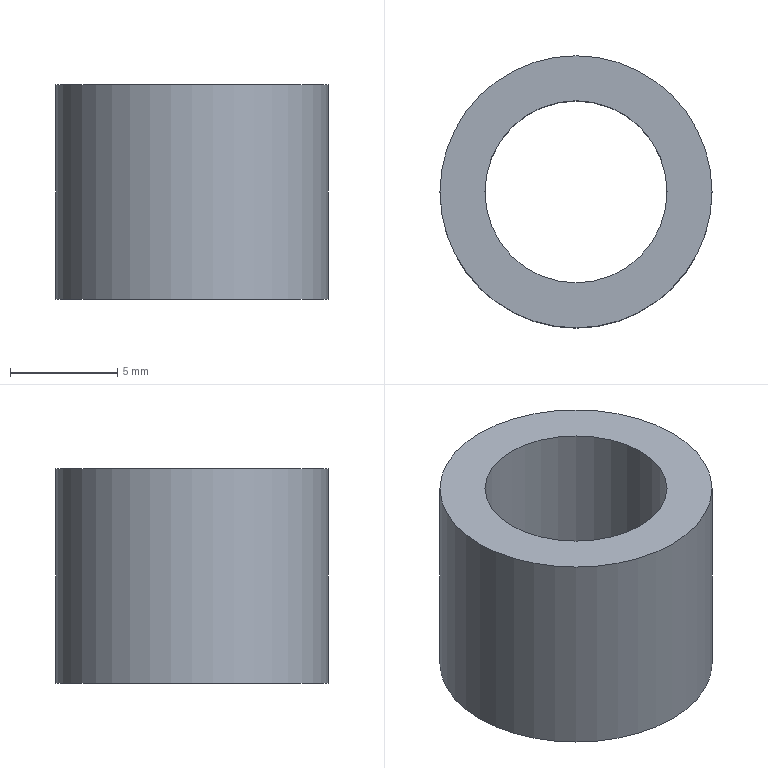Part | STEP file | 5091205 | 1 solid | 4 faces | box 12.7 x 12.7 x 10 mm | volume 699.319 mm3 | plane 2 | cylinder 2 | commonest cylinder face diameters 8.5 x1 12.7 x1
STEP:
#1=CARTESIAN_POINT('',(0.,0.,0.));
#2=DIRECTION('',(0.,0.,1.));
#3=DIRECTION('',(1.,0.,0.));
#4=AXIS2_PLACEMENT_3D('',#1,#2,#3);
#5=CARTESIAN_POINT('',(6.35,0.,5.));
#6=VERTEX_POINT('',#5);
#7=CARTESIAN_POINT('',(0.,0.,5.));
#8=DIRECTION('',(0.,0.,1.));
#9=DIRECTION('',(1.,0.,0.));
#10=AXIS2_PLACEMENT_3D('',#7,#8,#9);
#11=CIRCLE('',#10,6.35);
#12=CARTESIAN_POINT('',(0.,0.,5.));
#13=DIRECTION('',(0.,0.,1.));
#14=DIRECTION('',(1.,0.,0.));
#15=AXIS2_PLACEMENT_3D('',#12,#13,#14);
#16=PLANE('',#15);
#17=CARTESIAN_POINT('',(0.,0.));
#18=DIRECTION('',(1.,0.));
#19=AXIS2_PLACEMENT_2D('',#17,#18);
#20=CIRCLE('',#19,6.35);
#21=(GEOMETRIC_REPRESENTATION_CONTEXT(2)PARAMETRIC_REPRESENTATION_CONTEXT()REPRESENTATION_CONTEXT('',''));
#22=DEFINITIONAL_REPRESENTATION('',(#20),#21);
#23=PCURVE('',#16,#22);
#24=CARTESIAN_POINT('',(0.,0.,5.));
#25=DIRECTION('',(0.,0.,-1.));
#26=DIRECTION('',(-1.,0.,0.));
#27=AXIS2_PLACEMENT_3D('',#24,#25,#26);
#28=CYLINDRICAL_SURFACE('',#27,6.35);
#29=CARTESIAN_POINT('',(9.425,0.));
#30=DIRECTION('',(-1.,0.));
#31=VECTOR('',#30,1.);
#32=LINE('',#29,#31);
#33=(GEOMETRIC_REPRESENTATION_CONTEXT(2)PARAMETRIC_REPRESENTATION_CONTEXT()REPRESENTATION_CONTEXT('',''));
#34=DEFINITIONAL_REPRESENTATION('',(#32),#33);
#35=PCURVE('',#28,#34);
#36=SURFACE_CURVE('',#11,(#23,#35),.PCURVE_S1.);
#37=EDGE_CURVE('',#6,#6,#36,.T.);
#38=ORIENTED_EDGE('',*,*,#37,.T.);
#39=EDGE_LOOP('',(#38));
#40=FACE_BOUND('',#39,.T.);
#41=CARTESIAN_POINT('',(4.25,0.,5.));
#42=VERTEX_POINT('',#41);
#43=CARTESIAN_POINT('',(0.,0.,5.));
#44=DIRECTION('',(0.,0.,1.));
#45=DIRECTION('',(1.,0.,0.));
#46=AXIS2_PLACEMENT_3D('',#43,#44,#45);
#47=CIRCLE('',#46,4.25);
#48=CARTESIAN_POINT('',(0.,0.));
#49=DIRECTION('',(1.,0.));
#50=AXIS2_PLACEMENT_2D('',#48,#49);
#51=CIRCLE('',#50,4.25);
#52=(GEOMETRIC_REPRESENTATION_CONTEXT(2)PARAMETRIC_REPRESENTATION_CONTEXT()REPRESENTATION_CONTEXT('',''));
#53=DEFINITIONAL_REPRESENTATION('',(#51),#52);
#54=PCURVE('',#16,#53);
#55=CARTESIAN_POINT('',(0.,0.,5.));
#56=DIRECTION('',(0.,0.,-1.));
#57=DIRECTION('',(-1.,0.,0.));
#58=AXIS2_PLACEMENT_3D('',#55,#56,#57);
#59=CYLINDRICAL_SURFACE('',#58,4.25);
#60=CARTESIAN_POINT('',(9.425,0.));
#61=DIRECTION('',(-1.,0.));
#62=VECTOR('',#61,1.);
#63=LINE('',#60,#62);
#64=(GEOMETRIC_REPRESENTATION_CONTEXT(2)PARAMETRIC_REPRESENTATION_CONTEXT()REPRESENTATION_CONTEXT('',''));
#65=DEFINITIONAL_REPRESENTATION('',(#63),#64);
#66=PCURVE('',#59,#65);
#67=SURFACE_CURVE('',#47,(#54,#66),.PCURVE_S1.);
#68=EDGE_CURVE('',#42,#42,#67,.T.);
#69=ORIENTED_EDGE('',*,*,#68,.F.);
#70=EDGE_LOOP('',(#69));
#71=FACE_BOUND('',#70,.T.);
#72=ADVANCED_FACE('',(#40,#71),#16,.T.);
#73=CARTESIAN_POINT('',(6.35,0.,-5.));
#74=VERTEX_POINT('',#73);
#75=CARTESIAN_POINT('',(0.,0.,-5.));
#76=DIRECTION('',(0.,0.,1.));
#77=DIRECTION('',(1.,0.,0.));
#78=AXIS2_PLACEMENT_3D('',#75,#76,#77);
#79=CIRCLE('',#78,6.35);
#80=CARTESIAN_POINT('',(0.,0.,-5.));
#81=DIRECTION('',(0.,0.,1.));
#82=DIRECTION('',(1.,0.,0.));
#83=AXIS2_PLACEMENT_3D('',#80,#81,#82);
#84=PLANE('',#83);
#85=CARTESIAN_POINT('',(0.,0.));
#86=DIRECTION('',(1.,0.));
#87=AXIS2_PLACEMENT_2D('',#85,#86);
#88=CIRCLE('',#87,6.35);
#89=(GEOMETRIC_REPRESENTATION_CONTEXT(2)PARAMETRIC_REPRESENTATION_CONTEXT()REPRESENTATION_CONTEXT('',''));
#90=DEFINITIONAL_REPRESENTATION('',(#88),#89);
#91=PCURVE('',#84,#90);
#92=CARTESIAN_POINT('',(9.425,10.));
#93=DIRECTION('',(-1.,0.));
#94=VECTOR('',#93,1.);
#95=LINE('',#92,#94);
#96=(GEOMETRIC_REPRESENTATION_CONTEXT(2)PARAMETRIC_REPRESENTATION_CONTEXT()REPRESENTATION_CONTEXT('',''));
#97=DEFINITIONAL_REPRESENTATION('',(#95),#96);
#98=PCURVE('',#28,#97);
#99=SURFACE_CURVE('',#79,(#91,#98),.PCURVE_S1.);
#100=EDGE_CURVE('',#74,#74,#99,.T.);
#101=ORIENTED_EDGE('',*,*,#100,.F.);
#102=EDGE_LOOP('',(#101));
#103=FACE_BOUND('',#102,.T.);
#104=CARTESIAN_POINT('',(4.25,0.,-5.));
#105=VERTEX_POINT('',#104);
#106=CARTESIAN_POINT('',(0.,0.,-5.));
#107=DIRECTION('',(0.,0.,1.));
#108=DIRECTION('',(1.,0.,0.));
#109=AXIS2_PLACEMENT_3D('',#106,#107,#108);
#110=CIRCLE('',#109,4.25);
#111=CARTESIAN_POINT('',(0.,0.));
#112=DIRECTION('',(1.,0.));
#113=AXIS2_PLACEMENT_2D('',#111,#112);
#114=CIRCLE('',#113,4.25);
#115=(GEOMETRIC_REPRESENTATION_CONTEXT(2)PARAMETRIC_REPRESENTATION_CONTEXT()REPRESENTATION_CONTEXT('',''));
#116=DEFINITIONAL_REPRESENTATION('',(#114),#115);
#117=PCURVE('',#84,#116);
#118=CARTESIAN_POINT('',(9.425,10.));
#119=DIRECTION('',(-1.,0.));
#120=VECTOR('',#119,1.);
#121=LINE('',#118,#120);
#122=(GEOMETRIC_REPRESENTATION_CONTEXT(2)PARAMETRIC_REPRESENTATION_CONTEXT()REPRESENTATION_CONTEXT('',''));
#123=DEFINITIONAL_REPRESENTATION('',(#121),#122);
#124=PCURVE('',#59,#123);
#125=SURFACE_CURVE('',#110,(#117,#124),.PCURVE_S1.);
#126=EDGE_CURVE('',#105,#105,#125,.T.);
#127=ORIENTED_EDGE('',*,*,#126,.T.);
#128=EDGE_LOOP('',(#127));
#129=FACE_BOUND('',#128,.T.);
#130=ADVANCED_FACE('',(#103,#129),#84,.F.);
#131=ORIENTED_EDGE('',*,*,#37,.F.);
#132=CARTESIAN_POINT('',(6.35,0.,5.));
#133=CARTESIAN_POINT('',(6.35,0.,-5.));
#134=B_SPLINE_CURVE_WITH_KNOTS('',1,(#132,#133),.UNSPECIFIED.,.F.,.F.,(2,2),(0.,10.),.PIECEWISE_BEZIER_KNOTS.);
#135=CARTESIAN_POINT('',(9.425,0.));
#136=DIRECTION('',(0.,1.));
#137=VECTOR('',#136,1.);
#138=LINE('',#135,#137);
#139=(GEOMETRIC_REPRESENTATION_CONTEXT(2)PARAMETRIC_REPRESENTATION_CONTEXT()REPRESENTATION_CONTEXT('',''));
#140=DEFINITIONAL_REPRESENTATION('',(#138),#139);
#141=PCURVE('',#28,#140);
#142=CARTESIAN_POINT('',(3.142,0.));
#143=DIRECTION('',(0.,1.));
#144=VECTOR('',#143,1.);
#145=LINE('',#142,#144);
#146=(GEOMETRIC_REPRESENTATION_CONTEXT(2)PARAMETRIC_REPRESENTATION_CONTEXT()REPRESENTATION_CONTEXT('',''));
#147=DEFINITIONAL_REPRESENTATION('',(#145),#146);
#148=PCURVE('',#28,#147);
#149=SEAM_CURVE('',#134,(#141,#148),.PCURVE_S1.);
#150=EDGE_CURVE('',#6,#74,#149,.T.);
#151=ORIENTED_EDGE('',*,*,#150,.T.);
#152=ORIENTED_EDGE('',*,*,#100,.T.);
#153=ORIENTED_EDGE('',*,*,#150,.F.);
#154=EDGE_LOOP('',(#131,#151,#152,#153));
#155=FACE_BOUND('',#154,.T.);
#156=ADVANCED_FACE('',(#155),#28,.T.);
#157=ORIENTED_EDGE('',*,*,#68,.F.);
#158=CARTESIAN_POINT('',(4.25,0.,5.));
#159=CARTESIAN_POINT('',(4.25,0.,-5.));
#160=B_SPLINE_CURVE_WITH_KNOTS('',1,(#158,#159),.UNSPECIFIED.,.F.,.F.,(2,2),(0.,10.),.PIECEWISE_BEZIER_KNOTS.);
#161=CARTESIAN_POINT('',(9.425,0.));
#162=DIRECTION('',(0.,1.));
#163=VECTOR('',#162,1.);
#164=LINE('',#161,#163);
#165=(GEOMETRIC_REPRESENTATION_CONTEXT(2)PARAMETRIC_REPRESENTATION_CONTEXT()REPRESENTATION_CONTEXT('',''));
#166=DEFINITIONAL_REPRESENTATION('',(#164),#165);
#167=PCURVE('',#59,#166);
#168=CARTESIAN_POINT('',(3.142,0.));
#169=DIRECTION('',(0.,1.));
#170=VECTOR('',#169,1.);
#171=LINE('',#168,#170);
#172=(GEOMETRIC_REPRESENTATION_CONTEXT(2)PARAMETRIC_REPRESENTATION_CONTEXT()REPRESENTATION_CONTEXT('',''));
#173=DEFINITIONAL_REPRESENTATION('',(#171),#172);
#174=PCURVE('',#59,#173);
#175=SEAM_CURVE('',#160,(#167,#174),.PCURVE_S1.);
#176=EDGE_CURVE('',#42,#105,#175,.T.);
#177=ORIENTED_EDGE('',*,*,#176,.T.);
#178=ORIENTED_EDGE('',*,*,#126,.T.);
#179=ORIENTED_EDGE('',*,*,#176,.F.);
#180=EDGE_LOOP('',(#157,#177,#178,#179));
#181=FACE_BOUND('',#180,.F.);
#182=ADVANCED_FACE('',(#181),#59,.F.);
#183=CLOSED_SHELL('',(#72,#130,#156,#182));
#184=MANIFOLD_SOLID_BREP('',#183);
#185=(LENGTH_UNIT()NAMED_UNIT(*)SI_UNIT(.MILLI.,.METRE.));
#186=UNCERTAINTY_MEASURE_WITH_UNIT(LENGTH_MEASURE(0.00001),#185,'','');
#187=(NAMED_UNIT(*)PLANE_ANGLE_UNIT()SI_UNIT($,.RADIAN.));
#188=(NAMED_UNIT(*)SI_UNIT($,.STERADIAN.)SOLID_ANGLE_UNIT());
#189=(GEOMETRIC_REPRESENTATION_CONTEXT(3)GLOBAL_UNCERTAINTY_ASSIGNED_CONTEXT((#186))GLOBAL_UNIT_ASSIGNED_CONTEXT((#185,#187,#188))REPRESENTATION_CONTEXT('',''));
#190=ADVANCED_BREP_SHAPE_REPRESENTATION('',(#4,#184),#189);